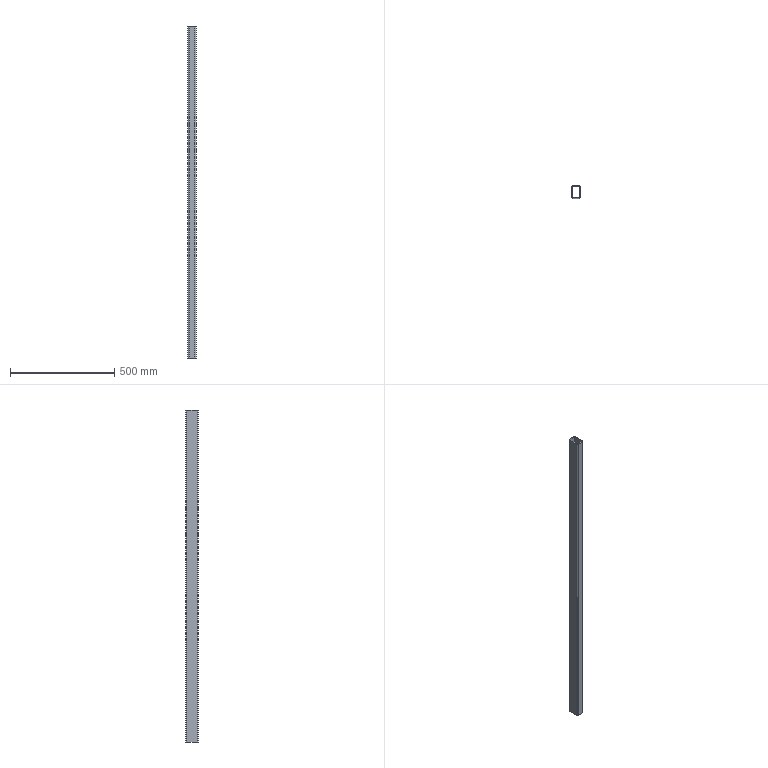Part | SolidWorks | features Cut 1, WeldMemberFeat 1, WeldmentFeature 1 | 1 solid | 18 faces | box 40 x 60 x 1590 mm | volume 859909 mm3 | plane 10 | cylinder 8 | commonest cylinder face diameters 6 x4 12 x4
STEP:
#1=CARTESIAN_POINT('',(-20.,24.,0.));
#2=VERTEX_POINT('',#1);
#3=CARTESIAN_POINT('',(-14.,30.,0.));
#4=VERTEX_POINT('',#3);
#5=CARTESIAN_POINT('',(-14.,24.,0.));
#6=DIRECTION('',(0.,0.,-1.));
#7=DIRECTION('',(-1.,0.,0.));
#8=AXIS2_PLACEMENT_3D('',#5,#6,#7);
#9=CIRCLE('',#8,6.);
#10=EDGE_CURVE('',#2,#4,#9,.T.);
#11=ORIENTED_EDGE('',*,*,#10,.T.);
#12=CARTESIAN_POINT('',(-14.,30.,-1590.));
#13=VERTEX_POINT('',#12);
#14=CARTESIAN_POINT('',(-14.,30.,-1590.));
#15=DIRECTION('',(0.,0.,1.));
#16=VECTOR('',#15,1000.);
#17=LINE('',#14,#16);
#18=EDGE_CURVE('',#13,#4,#17,.T.);
#19=ORIENTED_EDGE('',*,*,#18,.F.);
#20=CARTESIAN_POINT('',(-20.,24.,-1590.));
#21=VERTEX_POINT('',#20);
#22=CARTESIAN_POINT('',(-14.,24.,-1590.));
#23=DIRECTION('',(0.,0.,-1.));
#24=DIRECTION('',(-1.,0.,0.));
#25=AXIS2_PLACEMENT_3D('',#22,#23,#24);
#26=CIRCLE('',#25,6.);
#27=EDGE_CURVE('',#21,#13,#26,.T.);
#28=ORIENTED_EDGE('',*,*,#27,.F.);
#29=CARTESIAN_POINT('',(-20.,24.,-1590.));
#30=DIRECTION('',(0.,0.,1.));
#31=VECTOR('',#30,1000.);
#32=LINE('',#29,#31);
#33=EDGE_CURVE('',#21,#2,#32,.T.);
#34=ORIENTED_EDGE('',*,*,#33,.T.);
#35=EDGE_LOOP('',(#11,#19,#28,#34));
#36=FACE_OUTER_BOUND('',#35,.T.);
#37=CARTESIAN_POINT('',(-14.,24.,-1590.));
#38=DIRECTION('',(0.,0.,1.));
#39=DIRECTION('',(1.,0.,0.));
#40=AXIS2_PLACEMENT_3D('',#37,#38,#39);
#41=CYLINDRICAL_SURFACE('',#40,6.);
#42=ADVANCED_FACE('',(#36),#41,.T.);
#43=CARTESIAN_POINT('',(14.,30.,0.));
#44=VERTEX_POINT('',#43);
#45=CARTESIAN_POINT('',(-14.,30.,0.));
#46=DIRECTION('',(1.,0.,0.));
#47=VECTOR('',#46,1000.);
#48=LINE('',#45,#47);
#49=EDGE_CURVE('',#4,#44,#48,.T.);
#50=ORIENTED_EDGE('',*,*,#49,.T.);
#51=CARTESIAN_POINT('',(14.,30.,-1590.));
#52=VERTEX_POINT('',#51);
#53=CARTESIAN_POINT('',(14.,30.,-1590.));
#54=DIRECTION('',(0.,0.,1.));
#55=VECTOR('',#54,1000.);
#56=LINE('',#53,#55);
#57=EDGE_CURVE('',#52,#44,#56,.T.);
#58=ORIENTED_EDGE('',*,*,#57,.F.);
#59=CARTESIAN_POINT('',(-14.,30.,-1590.));
#60=DIRECTION('',(1.,0.,0.));
#61=VECTOR('',#60,1000.);
#62=LINE('',#59,#61);
#63=EDGE_CURVE('',#13,#52,#62,.T.);
#64=ORIENTED_EDGE('',*,*,#63,.F.);
#65=ORIENTED_EDGE('',*,*,#18,.T.);
#66=EDGE_LOOP('',(#50,#58,#64,#65));
#67=FACE_OUTER_BOUND('',#66,.T.);
#68=CARTESIAN_POINT('',(-14.,30.,-1590.));
#69=DIRECTION('',(0.,-1.,0.));
#70=DIRECTION('',(0.,0.,-1.));
#71=AXIS2_PLACEMENT_3D('',#68,#69,#70);
#72=PLANE('',#71);
#73=ADVANCED_FACE('',(#67),#72,.F.);
#74=CARTESIAN_POINT('',(20.,24.,0.));
#75=VERTEX_POINT('',#74);
#76=CARTESIAN_POINT('',(14.,24.,0.));
#77=DIRECTION('',(0.,0.,-1.));
#78=DIRECTION('',(-1.,0.,0.));
#79=AXIS2_PLACEMENT_3D('',#76,#77,#78);
#80=CIRCLE('',#79,6.);
#81=EDGE_CURVE('',#44,#75,#80,.T.);
#82=ORIENTED_EDGE('',*,*,#81,.T.);
#83=CARTESIAN_POINT('',(20.,24.,-1590.));
#84=VERTEX_POINT('',#83);
#85=CARTESIAN_POINT('',(20.,24.,-1590.));
#86=DIRECTION('',(0.,0.,1.));
#87=VECTOR('',#86,1000.);
#88=LINE('',#85,#87);
#89=EDGE_CURVE('',#84,#75,#88,.T.);
#90=ORIENTED_EDGE('',*,*,#89,.F.);
#91=CARTESIAN_POINT('',(14.,24.,-1590.));
#92=DIRECTION('',(0.,0.,-1.));
#93=DIRECTION('',(-1.,0.,0.));
#94=AXIS2_PLACEMENT_3D('',#91,#92,#93);
#95=CIRCLE('',#94,6.);
#96=EDGE_CURVE('',#52,#84,#95,.T.);
#97=ORIENTED_EDGE('',*,*,#96,.F.);
#98=ORIENTED_EDGE('',*,*,#57,.T.);
#99=EDGE_LOOP('',(#82,#90,#97,#98));
#100=FACE_OUTER_BOUND('',#99,.T.);
#101=CARTESIAN_POINT('',(14.,24.,-1590.));
#102=DIRECTION('',(0.,0.,1.));
#103=DIRECTION('',(1.,0.,0.));
#104=AXIS2_PLACEMENT_3D('',#101,#102,#103);
#105=CYLINDRICAL_SURFACE('',#104,6.);
#106=ADVANCED_FACE('',(#100),#105,.T.);
#107=CARTESIAN_POINT('',(20.,-24.,0.));
#108=VERTEX_POINT('',#107);
#109=CARTESIAN_POINT('',(20.,-24.,0.));
#110=DIRECTION('',(0.,-1.,0.));
#111=VECTOR('',#110,1000.);
#112=LINE('',#109,#111);
#113=EDGE_CURVE('',#75,#108,#112,.T.);
#114=ORIENTED_EDGE('',*,*,#113,.T.);
#115=CARTESIAN_POINT('',(20.,-24.,-1590.));
#116=VERTEX_POINT('',#115);
#117=CARTESIAN_POINT('',(20.,-24.,-1590.));
#118=DIRECTION('',(0.,0.,1.));
#119=VECTOR('',#118,1000.);
#120=LINE('',#117,#119);
#121=EDGE_CURVE('',#116,#108,#120,.T.);
#122=ORIENTED_EDGE('',*,*,#121,.F.);
#123=CARTESIAN_POINT('',(20.,-24.,-1590.));
#124=DIRECTION('',(0.,-1.,0.));
#125=VECTOR('',#124,1000.);
#126=LINE('',#123,#125);
#127=EDGE_CURVE('',#84,#116,#126,.T.);
#128=ORIENTED_EDGE('',*,*,#127,.F.);
#129=ORIENTED_EDGE('',*,*,#89,.T.);
#130=EDGE_LOOP('',(#114,#122,#128,#129));
#131=FACE_OUTER_BOUND('',#130,.T.);
#132=CARTESIAN_POINT('',(20.,-24.,-1590.));
#133=DIRECTION('',(-1.,0.,0.));
#134=DIRECTION('',(0.,0.,1.));
#135=AXIS2_PLACEMENT_3D('',#132,#133,#134);
#136=PLANE('',#135);
#137=ADVANCED_FACE('',(#131),#136,.F.);
#138=CARTESIAN_POINT('',(14.,-30.,0.));
#139=VERTEX_POINT('',#138);
#140=CARTESIAN_POINT('',(14.,-24.,0.));
#141=DIRECTION('',(0.,0.,-1.));
#142=DIRECTION('',(-1.,0.,0.));
#143=AXIS2_PLACEMENT_3D('',#140,#141,#142);
#144=CIRCLE('',#143,6.);
#145=EDGE_CURVE('',#108,#139,#144,.T.);
#146=ORIENTED_EDGE('',*,*,#145,.T.);
#147=CARTESIAN_POINT('',(14.,-30.,-1590.));
#148=VERTEX_POINT('',#147);
#149=CARTESIAN_POINT('',(14.,-30.,-1590.));
#150=DIRECTION('',(0.,0.,1.));
#151=VECTOR('',#150,1000.);
#152=LINE('',#149,#151);
#153=EDGE_CURVE('',#148,#139,#152,.T.);
#154=ORIENTED_EDGE('',*,*,#153,.F.);
#155=CARTESIAN_POINT('',(14.,-24.,-1590.));
#156=DIRECTION('',(0.,0.,-1.));
#157=DIRECTION('',(-1.,0.,0.));
#158=AXIS2_PLACEMENT_3D('',#155,#156,#157);
#159=CIRCLE('',#158,6.);
#160=EDGE_CURVE('',#116,#148,#159,.T.);
#161=ORIENTED_EDGE('',*,*,#160,.F.);
#162=ORIENTED_EDGE('',*,*,#121,.T.);
#163=EDGE_LOOP('',(#146,#154,#161,#162));
#164=FACE_OUTER_BOUND('',#163,.T.);
#165=CARTESIAN_POINT('',(14.,-24.,-1590.));
#166=DIRECTION('',(0.,0.,1.));
#167=DIRECTION('',(1.,0.,0.));
#168=AXIS2_PLACEMENT_3D('',#165,#166,#167);
#169=CYLINDRICAL_SURFACE('',#168,6.);
#170=ADVANCED_FACE('',(#164),#169,.T.);
#171=CARTESIAN_POINT('',(-14.,-30.,0.));
#172=VERTEX_POINT('',#171);
#173=CARTESIAN_POINT('',(14.,-30.,0.));
#174=DIRECTION('',(-1.,0.,0.));
#175=VECTOR('',#174,1000.);
#176=LINE('',#173,#175);
#177=EDGE_CURVE('',#139,#172,#176,.T.);
#178=ORIENTED_EDGE('',*,*,#177,.T.);
#179=CARTESIAN_POINT('',(-14.,-30.,-1590.));
#180=VERTEX_POINT('',#179);
#181=CARTESIAN_POINT('',(-14.,-30.,-1590.));
#182=DIRECTION('',(0.,0.,1.));
#183=VECTOR('',#182,1000.);
#184=LINE('',#181,#183);
#185=EDGE_CURVE('',#180,#172,#184,.T.);
#186=ORIENTED_EDGE('',*,*,#185,.F.);
#187=CARTESIAN_POINT('',(14.,-30.,-1590.));
#188=DIRECTION('',(-1.,0.,0.));
#189=VECTOR('',#188,1000.);
#190=LINE('',#187,#189);
#191=EDGE_CURVE('',#148,#180,#190,.T.);
#192=ORIENTED_EDGE('',*,*,#191,.F.);
#193=ORIENTED_EDGE('',*,*,#153,.T.);
#194=EDGE_LOOP('',(#178,#186,#192,#193));
#195=FACE_OUTER_BOUND('',#194,.T.);
#196=CARTESIAN_POINT('',(14.,-30.,-1590.));
#197=DIRECTION('',(0.,1.,0.));
#198=DIRECTION('',(0.,0.,1.));
#199=AXIS2_PLACEMENT_3D('',#196,#197,#198);
#200=PLANE('',#199);
#201=ADVANCED_FACE('',(#195),#200,.F.);
#202=CARTESIAN_POINT('',(-20.,-24.,0.));
#203=VERTEX_POINT('',#202);
#204=CARTESIAN_POINT('',(-14.,-24.,0.));
#205=DIRECTION('',(0.,0.,-1.));
#206=DIRECTION('',(-1.,0.,0.));
#207=AXIS2_PLACEMENT_3D('',#204,#205,#206);
#208=CIRCLE('',#207,6.);
#209=EDGE_CURVE('',#172,#203,#208,.T.);
#210=ORIENTED_EDGE('',*,*,#209,.T.);
#211=CARTESIAN_POINT('',(-20.,-24.,-1590.));
#212=VERTEX_POINT('',#211);
#213=CARTESIAN_POINT('',(-20.,-24.,-1590.));
#214=DIRECTION('',(0.,0.,1.));
#215=VECTOR('',#214,1000.);
#216=LINE('',#213,#215);
#217=EDGE_CURVE('',#212,#203,#216,.T.);
#218=ORIENTED_EDGE('',*,*,#217,.F.);
#219=CARTESIAN_POINT('',(-14.,-24.,-1590.));
#220=DIRECTION('',(0.,0.,-1.));
#221=DIRECTION('',(-1.,0.,0.));
#222=AXIS2_PLACEMENT_3D('',#219,#220,#221);
#223=CIRCLE('',#222,6.);
#224=EDGE_CURVE('',#180,#212,#223,.T.);
#225=ORIENTED_EDGE('',*,*,#224,.F.);
#226=ORIENTED_EDGE('',*,*,#185,.T.);
#227=EDGE_LOOP('',(#210,#218,#225,#226));
#228=FACE_OUTER_BOUND('',#227,.T.);
#229=CARTESIAN_POINT('',(-14.,-24.,-1590.));
#230=DIRECTION('',(0.,0.,1.));
#231=DIRECTION('',(1.,0.,0.));
#232=AXIS2_PLACEMENT_3D('',#229,#230,#231);
#233=CYLINDRICAL_SURFACE('',#232,6.);
#234=ADVANCED_FACE('',(#228),#233,.T.);
#235=CARTESIAN_POINT('',(14.,27.,0.));
#236=VERTEX_POINT('',#235);
#237=CARTESIAN_POINT('',(17.,24.,0.));
#238=VERTEX_POINT('',#237);
#239=CARTESIAN_POINT('',(14.,24.,0.));
#240=DIRECTION('',(0.,0.,-1.));
#241=DIRECTION('',(-1.,0.,0.));
#242=AXIS2_PLACEMENT_3D('',#239,#240,#241);
#243=CIRCLE('',#242,3.);
#244=EDGE_CURVE('',#236,#238,#243,.T.);
#245=ORIENTED_EDGE('',*,*,#244,.F.);
#246=CARTESIAN_POINT('',(14.,27.,-1590.));
#247=VERTEX_POINT('',#246);
#248=CARTESIAN_POINT('',(14.,27.,-1590.));
#249=DIRECTION('',(0.,0.,1.));
#250=VECTOR('',#249,1000.);
#251=LINE('',#248,#250);
#252=EDGE_CURVE('',#247,#236,#251,.T.);
#253=ORIENTED_EDGE('',*,*,#252,.F.);
#254=CARTESIAN_POINT('',(17.,24.,-1590.));
#255=VERTEX_POINT('',#254);
#256=CARTESIAN_POINT('',(14.,24.,-1590.));
#257=DIRECTION('',(0.,0.,-1.));
#258=DIRECTION('',(-1.,0.,0.));
#259=AXIS2_PLACEMENT_3D('',#256,#257,#258);
#260=CIRCLE('',#259,3.);
#261=EDGE_CURVE('',#247,#255,#260,.T.);
#262=ORIENTED_EDGE('',*,*,#261,.T.);
#263=CARTESIAN_POINT('',(17.,24.,-1590.));
#264=DIRECTION('',(0.,0.,1.));
#265=VECTOR('',#264,1000.);
#266=LINE('',#263,#265);
#267=EDGE_CURVE('',#255,#238,#266,.T.);
#268=ORIENTED_EDGE('',*,*,#267,.T.);
#269=EDGE_LOOP('',(#245,#253,#262,#268));
#270=FACE_OUTER_BOUND('',#269,.T.);
#271=CARTESIAN_POINT('',(14.,24.,-1590.));
#272=DIRECTION('',(0.,0.,1.));
#273=DIRECTION('',(1.,0.,0.));
#274=AXIS2_PLACEMENT_3D('',#271,#272,#273);
#275=CYLINDRICAL_SURFACE('',#274,3.);
#276=ADVANCED_FACE('',(#270),#275,.F.);
#277=CARTESIAN_POINT('',(-14.,27.,0.));
#278=VERTEX_POINT('',#277);
#279=CARTESIAN_POINT('',(-14.,27.,0.));
#280=DIRECTION('',(1.,0.,0.));
#281=VECTOR('',#280,1000.);
#282=LINE('',#279,#281);
#283=EDGE_CURVE('',#278,#236,#282,.T.);
#284=ORIENTED_EDGE('',*,*,#283,.F.);
#285=CARTESIAN_POINT('',(-14.,27.,-1590.));
#286=VERTEX_POINT('',#285);
#287=CARTESIAN_POINT('',(-14.,27.,-1590.));
#288=DIRECTION('',(0.,0.,1.));
#289=VECTOR('',#288,1000.);
#290=LINE('',#287,#289);
#291=EDGE_CURVE('',#286,#278,#290,.T.);
#292=ORIENTED_EDGE('',*,*,#291,.F.);
#293=CARTESIAN_POINT('',(-14.,27.,-1590.));
#294=DIRECTION('',(1.,0.,0.));
#295=VECTOR('',#294,1000.);
#296=LINE('',#293,#295);
#297=EDGE_CURVE('',#286,#247,#296,.T.);
#298=ORIENTED_EDGE('',*,*,#297,.T.);
#299=ORIENTED_EDGE('',*,*,#252,.T.);
#300=EDGE_LOOP('',(#284,#292,#298,#299));
#301=FACE_OUTER_BOUND('',#300,.T.);
#302=CARTESIAN_POINT('',(-14.,27.,-1590.));
#303=DIRECTION('',(0.,-1.,0.));
#304=DIRECTION('',(0.,0.,-1.));
#305=AXIS2_PLACEMENT_3D('',#302,#303,#304);
#306=PLANE('',#305);
#307=ADVANCED_FACE('',(#301),#306,.T.);
#308=CARTESIAN_POINT('',(-17.,24.,0.));
#309=VERTEX_POINT('',#308);
#310=CARTESIAN_POINT('',(-14.,24.,0.));
#311=DIRECTION('',(0.,0.,-1.));
#312=DIRECTION('',(-1.,0.,0.));
#313=AXIS2_PLACEMENT_3D('',#310,#311,#312);
#314=CIRCLE('',#313,3.);
#315=EDGE_CURVE('',#309,#278,#314,.T.);
#316=ORIENTED_EDGE('',*,*,#315,.F.);
#317=CARTESIAN_POINT('',(-17.,24.,-1590.));
#318=VERTEX_POINT('',#317);
#319=CARTESIAN_POINT('',(-17.,24.,-1590.));
#320=DIRECTION('',(0.,0.,1.));
#321=VECTOR('',#320,1000.);
#322=LINE('',#319,#321);
#323=EDGE_CURVE('',#318,#309,#322,.T.);
#324=ORIENTED_EDGE('',*,*,#323,.F.);
#325=CARTESIAN_POINT('',(-14.,24.,-1590.));
#326=DIRECTION('',(0.,0.,-1.));
#327=DIRECTION('',(-1.,0.,0.));
#328=AXIS2_PLACEMENT_3D('',#325,#326,#327);
#329=CIRCLE('',#328,3.);
#330=EDGE_CURVE('',#318,#286,#329,.T.);
#331=ORIENTED_EDGE('',*,*,#330,.T.);
#332=ORIENTED_EDGE('',*,*,#291,.T.);
#333=EDGE_LOOP('',(#316,#324,#331,#332));
#334=FACE_OUTER_BOUND('',#333,.T.);
#335=CARTESIAN_POINT('',(-14.,24.,-1590.));
#336=DIRECTION('',(0.,0.,1.));
#337=DIRECTION('',(1.,0.,0.));
#338=AXIS2_PLACEMENT_3D('',#335,#336,#337);
#339=CYLINDRICAL_SURFACE('',#338,3.);
#340=ADVANCED_FACE('',(#334),#339,.F.);
#341=CARTESIAN_POINT('',(-17.,-24.,0.));
#342=VERTEX_POINT('',#341);
#343=CARTESIAN_POINT('',(-17.,24.,0.));
#344=DIRECTION('',(0.,1.,0.));
#345=VECTOR('',#344,1000.);
#346=LINE('',#343,#345);
#347=EDGE_CURVE('',#342,#309,#346,.T.);
#348=ORIENTED_EDGE('',*,*,#347,.F.);
#349=CARTESIAN_POINT('',(-17.,-24.,-1590.));
#350=VERTEX_POINT('',#349);
#351=CARTESIAN_POINT('',(-17.,-24.,-1590.));
#352=DIRECTION('',(0.,0.,1.));
#353=VECTOR('',#352,1000.);
#354=LINE('',#351,#353);
#355=EDGE_CURVE('',#350,#342,#354,.T.);
#356=ORIENTED_EDGE('',*,*,#355,.F.);
#357=CARTESIAN_POINT('',(-17.,24.,-1590.));
#358=DIRECTION('',(0.,1.,0.));
#359=VECTOR('',#358,1000.);
#360=LINE('',#357,#359);
#361=EDGE_CURVE('',#350,#318,#360,.T.);
#362=ORIENTED_EDGE('',*,*,#361,.T.);
#363=ORIENTED_EDGE('',*,*,#323,.T.);
#364=EDGE_LOOP('',(#348,#356,#362,#363));
#365=FACE_OUTER_BOUND('',#364,.T.);
#366=CARTESIAN_POINT('',(-17.,24.,-1590.));
#367=DIRECTION('',(1.,0.,0.));
#368=DIRECTION('',(0.,0.,-1.));
#369=AXIS2_PLACEMENT_3D('',#366,#367,#368);
#370=PLANE('',#369);
#371=ADVANCED_FACE('',(#365),#370,.T.);
#372=CARTESIAN_POINT('',(-14.,-27.,0.));
#373=VERTEX_POINT('',#372);
#374=CARTESIAN_POINT('',(-14.,-24.,0.));
#375=DIRECTION('',(0.,0.,-1.));
#376=DIRECTION('',(-1.,0.,0.));
#377=AXIS2_PLACEMENT_3D('',#374,#375,#376);
#378=CIRCLE('',#377,3.);
#379=EDGE_CURVE('',#373,#342,#378,.T.);
#380=ORIENTED_EDGE('',*,*,#379,.F.);
#381=CARTESIAN_POINT('',(-14.,-27.,-1590.));
#382=VERTEX_POINT('',#381);
#383=CARTESIAN_POINT('',(-14.,-27.,-1590.));
#384=DIRECTION('',(0.,0.,1.));
#385=VECTOR('',#384,1000.);
#386=LINE('',#383,#385);
#387=EDGE_CURVE('',#382,#373,#386,.T.);
#388=ORIENTED_EDGE('',*,*,#387,.F.);
#389=CARTESIAN_POINT('',(-14.,-24.,-1590.));
#390=DIRECTION('',(0.,0.,-1.));
#391=DIRECTION('',(-1.,0.,0.));
#392=AXIS2_PLACEMENT_3D('',#389,#390,#391);
#393=CIRCLE('',#392,3.);
#394=EDGE_CURVE('',#382,#350,#393,.T.);
#395=ORIENTED_EDGE('',*,*,#394,.T.);
#396=ORIENTED_EDGE('',*,*,#355,.T.);
#397=EDGE_LOOP('',(#380,#388,#395,#396));
#398=FACE_OUTER_BOUND('',#397,.T.);
#399=CARTESIAN_POINT('',(-14.,-24.,-1590.));
#400=DIRECTION('',(0.,0.,1.));
#401=DIRECTION('',(1.,0.,0.));
#402=AXIS2_PLACEMENT_3D('',#399,#400,#401);
#403=CYLINDRICAL_SURFACE('',#402,3.);
#404=ADVANCED_FACE('',(#398),#403,.F.);
#405=CARTESIAN_POINT('',(14.,-27.,0.));
#406=VERTEX_POINT('',#405);
#407=CARTESIAN_POINT('',(14.,-27.,0.));
#408=DIRECTION('',(-1.,0.,0.));
#409=VECTOR('',#408,1000.);
#410=LINE('',#407,#409);
#411=EDGE_CURVE('',#406,#373,#410,.T.);
#412=ORIENTED_EDGE('',*,*,#411,.F.);
#413=CARTESIAN_POINT('',(14.,-27.,-1590.));
#414=VERTEX_POINT('',#413);
#415=CARTESIAN_POINT('',(14.,-27.,-1590.));
#416=DIRECTION('',(0.,0.,1.));
#417=VECTOR('',#416,1000.);
#418=LINE('',#415,#417);
#419=EDGE_CURVE('',#414,#406,#418,.T.);
#420=ORIENTED_EDGE('',*,*,#419,.F.);
#421=CARTESIAN_POINT('',(14.,-27.,-1590.));
#422=DIRECTION('',(-1.,0.,0.));
#423=VECTOR('',#422,1000.);
#424=LINE('',#421,#423);
#425=EDGE_CURVE('',#414,#382,#424,.T.);
#426=ORIENTED_EDGE('',*,*,#425,.T.);
#427=ORIENTED_EDGE('',*,*,#387,.T.);
#428=EDGE_LOOP('',(#412,#420,#426,#427));
#429=FACE_OUTER_BOUND('',#428,.T.);
#430=CARTESIAN_POINT('',(14.,-27.,-1590.));
#431=DIRECTION('',(0.,1.,0.));
#432=DIRECTION('',(0.,0.,1.));
#433=AXIS2_PLACEMENT_3D('',#430,#431,#432);
#434=PLANE('',#433);
#435=ADVANCED_FACE('',(#429),#434,.T.);
#436=CARTESIAN_POINT('',(17.,-24.,0.));
#437=VERTEX_POINT('',#436);
#438=CARTESIAN_POINT('',(14.,-24.,0.));
#439=DIRECTION('',(0.,0.,-1.));
#440=DIRECTION('',(-1.,0.,0.));
#441=AXIS2_PLACEMENT_3D('',#438,#439,#440);
#442=CIRCLE('',#441,3.);
#443=EDGE_CURVE('',#437,#406,#442,.T.);
#444=ORIENTED_EDGE('',*,*,#443,.F.);
#445=CARTESIAN_POINT('',(17.,-24.,-1590.));
#446=VERTEX_POINT('',#445);
#447=CARTESIAN_POINT('',(17.,-24.,-1590.));
#448=DIRECTION('',(0.,0.,1.));
#449=VECTOR('',#448,1000.);
#450=LINE('',#447,#449);
#451=EDGE_CURVE('',#446,#437,#450,.T.);
#452=ORIENTED_EDGE('',*,*,#451,.F.);
#453=CARTESIAN_POINT('',(14.,-24.,-1590.));
#454=DIRECTION('',(0.,0.,-1.));
#455=DIRECTION('',(-1.,0.,0.));
#456=AXIS2_PLACEMENT_3D('',#453,#454,#455);
#457=CIRCLE('',#456,3.);
#458=EDGE_CURVE('',#446,#414,#457,.T.);
#459=ORIENTED_EDGE('',*,*,#458,.T.);
#460=ORIENTED_EDGE('',*,*,#419,.T.);
#461=EDGE_LOOP('',(#444,#452,#459,#460));
#462=FACE_OUTER_BOUND('',#461,.T.);
#463=CARTESIAN_POINT('',(14.,-24.,-1590.));
#464=DIRECTION('',(0.,0.,1.));
#465=DIRECTION('',(1.,0.,0.));
#466=AXIS2_PLACEMENT_3D('',#463,#464,#465);
#467=CYLINDRICAL_SURFACE('',#466,3.);
#468=ADVANCED_FACE('',(#462),#467,.F.);
#469=CARTESIAN_POINT('',(17.,-24.,0.));
#470=DIRECTION('',(0.,-1.,0.));
#471=VECTOR('',#470,1000.);
#472=LINE('',#469,#471);
#473=EDGE_CURVE('',#238,#437,#472,.T.);
#474=ORIENTED_EDGE('',*,*,#473,.F.);
#475=ORIENTED_EDGE('',*,*,#267,.F.);
#476=CARTESIAN_POINT('',(17.,-24.,-1590.));
#477=DIRECTION('',(0.,-1.,0.));
#478=VECTOR('',#477,1000.);
#479=LINE('',#476,#478);
#480=EDGE_CURVE('',#255,#446,#479,.T.);
#481=ORIENTED_EDGE('',*,*,#480,.T.);
#482=ORIENTED_EDGE('',*,*,#451,.T.);
#483=EDGE_LOOP('',(#474,#475,#481,#482));
#484=FACE_OUTER_BOUND('',#483,.T.);
#485=CARTESIAN_POINT('',(17.,-24.,-1590.));
#486=DIRECTION('',(-1.,0.,0.));
#487=DIRECTION('',(0.,0.,1.));
#488=AXIS2_PLACEMENT_3D('',#485,#486,#487);
#489=PLANE('',#488);
#490=ADVANCED_FACE('',(#484),#489,.T.);
#491=CARTESIAN_POINT('',(-20.,24.,0.));
#492=DIRECTION('',(0.,1.,0.));
#493=VECTOR('',#492,1000.);
#494=LINE('',#491,#493);
#495=EDGE_CURVE('',#203,#2,#494,.T.);
#496=ORIENTED_EDGE('',*,*,#495,.T.);
#497=ORIENTED_EDGE('',*,*,#33,.F.);
#498=CARTESIAN_POINT('',(-20.,24.,-1590.));
#499=DIRECTION('',(0.,1.,0.));
#500=VECTOR('',#499,1000.);
#501=LINE('',#498,#500);
#502=EDGE_CURVE('',#212,#21,#501,.T.);
#503=ORIENTED_EDGE('',*,*,#502,.F.);
#504=ORIENTED_EDGE('',*,*,#217,.T.);
#505=EDGE_LOOP('',(#496,#497,#503,#504));
#506=FACE_OUTER_BOUND('',#505,.T.);
#507=CARTESIAN_POINT('',(-20.,24.,-1590.));
#508=DIRECTION('',(1.,0.,0.));
#509=DIRECTION('',(0.,0.,-1.));
#510=AXIS2_PLACEMENT_3D('',#507,#508,#509);
#511=PLANE('',#510);
#512=ADVANCED_FACE('',(#506),#511,.F.);
#513=ORIENTED_EDGE('',*,*,#261,.F.);
#514=ORIENTED_EDGE('',*,*,#297,.F.);
#515=ORIENTED_EDGE('',*,*,#330,.F.);
#516=ORIENTED_EDGE('',*,*,#361,.F.);
#517=ORIENTED_EDGE('',*,*,#394,.F.);
#518=ORIENTED_EDGE('',*,*,#425,.F.);
#519=ORIENTED_EDGE('',*,*,#458,.F.);
#520=ORIENTED_EDGE('',*,*,#480,.F.);
#521=EDGE_LOOP('',(#513,#514,#515,#516,#517,#518,#519,#520));
#522=FACE_BOUND('',#521,.T.);
#523=ORIENTED_EDGE('',*,*,#27,.T.);
#524=ORIENTED_EDGE('',*,*,#63,.T.);
#525=ORIENTED_EDGE('',*,*,#96,.T.);
#526=ORIENTED_EDGE('',*,*,#127,.T.);
#527=ORIENTED_EDGE('',*,*,#160,.T.);
#528=ORIENTED_EDGE('',*,*,#191,.T.);
#529=ORIENTED_EDGE('',*,*,#224,.T.);
#530=ORIENTED_EDGE('',*,*,#502,.T.);
#531=EDGE_LOOP('',(#523,#524,#525,#526,#527,#528,#529,#530));
#532=FACE_OUTER_BOUND('',#531,.T.);
#533=CARTESIAN_POINT('',(-14.,24.,-1590.));
#534=DIRECTION('',(0.,0.,-1.));
#535=DIRECTION('',(-1.,0.,0.));
#536=AXIS2_PLACEMENT_3D('',#533,#534,#535);
#537=PLANE('',#536);
#538=ADVANCED_FACE('',(#522,#532),#537,.T.);
#539=ORIENTED_EDGE('',*,*,#244,.T.);
#540=ORIENTED_EDGE('',*,*,#473,.T.);
#541=ORIENTED_EDGE('',*,*,#443,.T.);
#542=ORIENTED_EDGE('',*,*,#411,.T.);
#543=ORIENTED_EDGE('',*,*,#379,.T.);
#544=ORIENTED_EDGE('',*,*,#347,.T.);
#545=ORIENTED_EDGE('',*,*,#315,.T.);
#546=ORIENTED_EDGE('',*,*,#283,.T.);
#547=EDGE_LOOP('',(#539,#540,#541,#542,#543,#544,#545,#546));
#548=FACE_BOUND('',#547,.T.);
#549=ORIENTED_EDGE('',*,*,#10,.F.);
#550=ORIENTED_EDGE('',*,*,#495,.F.);
#551=ORIENTED_EDGE('',*,*,#209,.F.);
#552=ORIENTED_EDGE('',*,*,#177,.F.);
#553=ORIENTED_EDGE('',*,*,#145,.F.);
#554=ORIENTED_EDGE('',*,*,#113,.F.);
#555=ORIENTED_EDGE('',*,*,#81,.F.);
#556=ORIENTED_EDGE('',*,*,#49,.F.);
#557=EDGE_LOOP('',(#549,#550,#551,#552,#553,#554,#555,#556));
#558=FACE_OUTER_BOUND('',#557,.T.);
#559=CARTESIAN_POINT('',(-14.,24.,0.));
#560=DIRECTION('',(0.,0.,-1.));
#561=DIRECTION('',(-1.,0.,0.));
#562=AXIS2_PLACEMENT_3D('',#559,#560,#561);
#563=PLANE('',#562);
#564=ADVANCED_FACE('',(#548,#558),#563,.F.);
#565=CLOSED_SHELL('',(#42,#73,#106,#137,#170,#201,#234,#276,#307,#340,#371,#404,#435,#468,#490,#512,#538,#564));
#566=MANIFOLD_SOLID_BREP('',#565);
#567=CARTESIAN_POINT('',(0.,0.,0.));
#568=DIRECTION('',(0.,0.,1.));
#569=DIRECTION('',(1.,0.,0.));
#570=AXIS2_PLACEMENT_3D('',#567,#568,#569);
#571=(LENGTH_UNIT()NAMED_UNIT(*)SI_UNIT(.MILLI.,.METRE.));
#572=UNCERTAINTY_MEASURE_WITH_UNIT(LENGTH_MEASURE(0.00001),#571,'','');
#573=(NAMED_UNIT(*)PLANE_ANGLE_UNIT()SI_UNIT($,.RADIAN.));
#574=(NAMED_UNIT(*)SI_UNIT($,.STERADIAN.)SOLID_ANGLE_UNIT());
#575=(GEOMETRIC_REPRESENTATION_CONTEXT(3)GLOBAL_UNCERTAINTY_ASSIGNED_CONTEXT((#572))GLOBAL_UNIT_ASSIGNED_CONTEXT((#571,#573,#574))REPRESENTATION_CONTEXT('',''));
#576=ADVANCED_BREP_SHAPE_REPRESENTATION('',(#566,#570),#575);